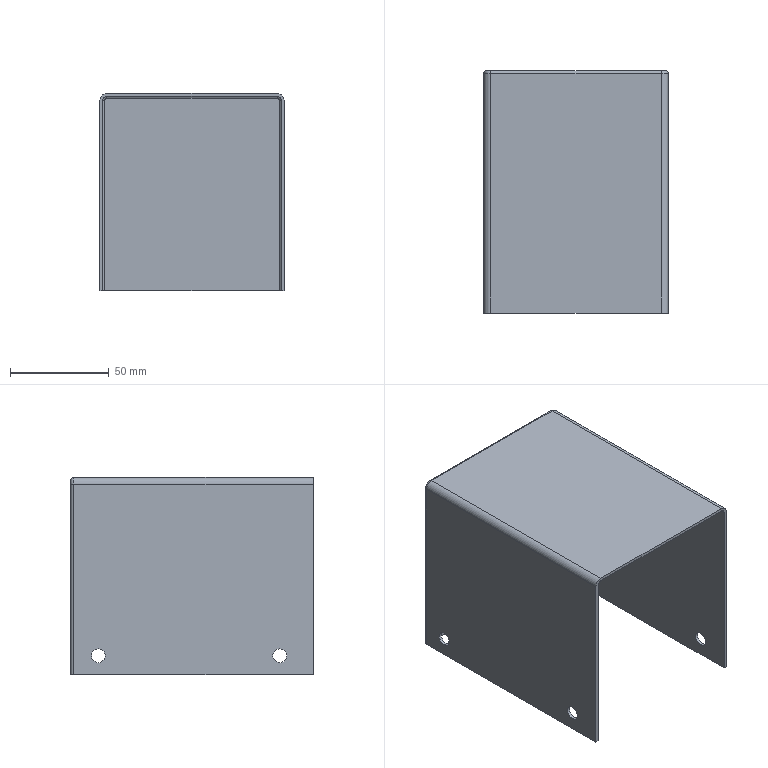Part | SolidWorks | features Fillet 4, Cut 2, Extrusion 1, ICE 1 | 1 solid | 32 faces | box 93.5 x 123 x 100 mm | volume 66221 mm3 | cylinder 18 | plane 10 | torus 4 | commonest cylinder face diameters 7 x10 2 x3 3 x3 4 x2
STEP:
#1=CARTESIAN_POINT('',(45.25,47.5,6.));
#2=VERTEX_POINT('',#1);
#3=CARTESIAN_POINT('',(45.25,47.5,13.));
#4=VERTEX_POINT('',#3);
#5=CARTESIAN_POINT('',(45.25,47.5,9.5));
#6=DIRECTION('',(-1.,0.,0.));
#7=DIRECTION('',(0.,0.,1.));
#8=AXIS2_PLACEMENT_3D('',#5,#6,#7);
#9=CIRCLE('',#8,3.5);
#10=EDGE_CURVE('',#2,#4,#9,.T.);
#11=ORIENTED_EDGE('',*,*,#10,.T.);
#12=CARTESIAN_POINT('',(46.75,47.5,13.));
#13=VERTEX_POINT('',#12);
#14=CARTESIAN_POINT('',(-46.75,47.5,13.));
#15=DIRECTION('',(1.,0.,0.));
#16=VECTOR('',#15,1000.);
#17=LINE('',#14,#16);
#18=EDGE_CURVE('',#4,#13,#17,.T.);
#19=ORIENTED_EDGE('',*,*,#18,.T.);
#20=CARTESIAN_POINT('',(46.75,47.5,6.));
#21=VERTEX_POINT('',#20);
#22=CARTESIAN_POINT('',(46.75,47.5,9.5));
#23=DIRECTION('',(1.,0.,0.));
#24=DIRECTION('',(0.,0.,-1.));
#25=AXIS2_PLACEMENT_3D('',#22,#23,#24);
#26=CIRCLE('',#25,3.5);
#27=EDGE_CURVE('',#13,#21,#26,.T.);
#28=ORIENTED_EDGE('',*,*,#27,.T.);
#29=CARTESIAN_POINT('',(-46.75,47.5,6.));
#30=DIRECTION('',(1.,0.,0.));
#31=VECTOR('',#30,1000.);
#32=LINE('',#29,#31);
#33=EDGE_CURVE('',#2,#21,#32,.T.);
#34=ORIENTED_EDGE('',*,*,#33,.F.);
#35=EDGE_LOOP('',(#11,#19,#28,#34));
#36=FACE_OUTER_BOUND('',#35,.T.);
#37=CARTESIAN_POINT('',(-46.75,47.5,9.5));
#38=DIRECTION('',(1.,0.,0.));
#39=DIRECTION('',(0.,0.,-1.));
#40=AXIS2_PLACEMENT_3D('',#37,#38,#39);
#41=CYLINDRICAL_SURFACE('',#40,3.5);
#42=ADVANCED_FACE('',(#36),#41,.F.);
#43=CARTESIAN_POINT('',(-46.75,47.5,13.));
#44=VERTEX_POINT('',#43);
#45=CARTESIAN_POINT('',(-46.75,47.5,6.));
#46=VERTEX_POINT('',#45);
#47=CARTESIAN_POINT('',(-46.75,47.5,9.5));
#48=DIRECTION('',(1.,0.,0.));
#49=DIRECTION('',(0.,0.,-1.));
#50=AXIS2_PLACEMENT_3D('',#47,#48,#49);
#51=CIRCLE('',#50,3.5);
#52=EDGE_CURVE('',#44,#46,#51,.T.);
#53=ORIENTED_EDGE('',*,*,#52,.F.);
#54=CARTESIAN_POINT('',(-45.25,47.5,13.));
#55=VERTEX_POINT('',#54);
#56=CARTESIAN_POINT('',(-46.75,47.5,13.));
#57=DIRECTION('',(1.,0.,0.));
#58=VECTOR('',#57,1000.);
#59=LINE('',#56,#58);
#60=EDGE_CURVE('',#44,#55,#59,.T.);
#61=ORIENTED_EDGE('',*,*,#60,.T.);
#62=CARTESIAN_POINT('',(-45.25,47.5,6.));
#63=VERTEX_POINT('',#62);
#64=CARTESIAN_POINT('',(-45.25,47.5,9.5));
#65=DIRECTION('',(1.,0.,0.));
#66=DIRECTION('',(0.,1.,0.));
#67=AXIS2_PLACEMENT_3D('',#64,#65,#66);
#68=CIRCLE('',#67,3.5);
#69=EDGE_CURVE('',#55,#63,#68,.T.);
#70=ORIENTED_EDGE('',*,*,#69,.T.);
#71=CARTESIAN_POINT('',(-46.75,47.5,6.));
#72=DIRECTION('',(1.,0.,0.));
#73=VECTOR('',#72,1000.);
#74=LINE('',#71,#73);
#75=EDGE_CURVE('',#46,#63,#74,.T.);
#76=ORIENTED_EDGE('',*,*,#75,.F.);
#77=EDGE_LOOP('',(#53,#61,#70,#76));
#78=FACE_OUTER_BOUND('',#77,.T.);
#79=CARTESIAN_POINT('',(-46.75,47.5,9.5));
#80=DIRECTION('',(1.,0.,0.));
#81=DIRECTION('',(0.,0.,-1.));
#82=AXIS2_PLACEMENT_3D('',#79,#80,#81);
#83=CYLINDRICAL_SURFACE('',#82,3.5);
#84=ADVANCED_FACE('',(#78),#83,.F.);
#85=CARTESIAN_POINT('',(45.25,-44.5,6.));
#86=VERTEX_POINT('',#85);
#87=CARTESIAN_POINT('',(45.25,-44.5,13.));
#88=VERTEX_POINT('',#87);
#89=CARTESIAN_POINT('',(45.25,-44.5,9.5));
#90=DIRECTION('',(-1.,0.,0.));
#91=DIRECTION('',(0.,0.,1.));
#92=AXIS2_PLACEMENT_3D('',#89,#90,#91);
#93=CIRCLE('',#92,3.5);
#94=EDGE_CURVE('',#86,#88,#93,.T.);
#95=ORIENTED_EDGE('',*,*,#94,.T.);
#96=CARTESIAN_POINT('',(46.75,-44.5,13.));
#97=VERTEX_POINT('',#96);
#98=CARTESIAN_POINT('',(-46.75,-44.5,13.));
#99=DIRECTION('',(1.,0.,0.));
#100=VECTOR('',#99,1000.);
#101=LINE('',#98,#100);
#102=EDGE_CURVE('',#88,#97,#101,.T.);
#103=ORIENTED_EDGE('',*,*,#102,.T.);
#104=CARTESIAN_POINT('',(46.75,-44.5,6.));
#105=VERTEX_POINT('',#104);
#106=CARTESIAN_POINT('',(46.75,-44.5,9.5));
#107=DIRECTION('',(1.,0.,0.));
#108=DIRECTION('',(0.,0.,-1.));
#109=AXIS2_PLACEMENT_3D('',#106,#107,#108);
#110=CIRCLE('',#109,3.5);
#111=EDGE_CURVE('',#97,#105,#110,.T.);
#112=ORIENTED_EDGE('',*,*,#111,.T.);
#113=CARTESIAN_POINT('',(-46.75,-44.5,6.));
#114=DIRECTION('',(1.,0.,0.));
#115=VECTOR('',#114,1000.);
#116=LINE('',#113,#115);
#117=EDGE_CURVE('',#86,#105,#116,.T.);
#118=ORIENTED_EDGE('',*,*,#117,.F.);
#119=EDGE_LOOP('',(#95,#103,#112,#118));
#120=FACE_OUTER_BOUND('',#119,.T.);
#121=CARTESIAN_POINT('',(-46.75,-44.5,9.5));
#122=DIRECTION('',(1.,0.,0.));
#123=DIRECTION('',(0.,0.,-1.));
#124=AXIS2_PLACEMENT_3D('',#121,#122,#123);
#125=CYLINDRICAL_SURFACE('',#124,3.5);
#126=ADVANCED_FACE('',(#120),#125,.F.);
#127=CARTESIAN_POINT('',(-46.75,-44.5,13.));
#128=VERTEX_POINT('',#127);
#129=CARTESIAN_POINT('',(-46.75,-44.5,6.));
#130=VERTEX_POINT('',#129);
#131=CARTESIAN_POINT('',(-46.75,-44.5,9.5));
#132=DIRECTION('',(1.,0.,0.));
#133=DIRECTION('',(0.,0.,-1.));
#134=AXIS2_PLACEMENT_3D('',#131,#132,#133);
#135=CIRCLE('',#134,3.5);
#136=EDGE_CURVE('',#128,#130,#135,.T.);
#137=ORIENTED_EDGE('',*,*,#136,.F.);
#138=CARTESIAN_POINT('',(-45.25,-44.5,13.));
#139=VERTEX_POINT('',#138);
#140=CARTESIAN_POINT('',(-46.75,-44.5,13.));
#141=DIRECTION('',(1.,0.,0.));
#142=VECTOR('',#141,1000.);
#143=LINE('',#140,#142);
#144=EDGE_CURVE('',#128,#139,#143,.T.);
#145=ORIENTED_EDGE('',*,*,#144,.T.);
#146=CARTESIAN_POINT('',(-45.25,-44.5,6.));
#147=VERTEX_POINT('',#146);
#148=CARTESIAN_POINT('',(-45.25,-44.5,9.5));
#149=DIRECTION('',(1.,0.,0.));
#150=DIRECTION('',(0.,1.,0.));
#151=AXIS2_PLACEMENT_3D('',#148,#149,#150);
#152=CIRCLE('',#151,3.5);
#153=EDGE_CURVE('',#139,#147,#152,.T.);
#154=ORIENTED_EDGE('',*,*,#153,.T.);
#155=CARTESIAN_POINT('',(-46.75,-44.5,6.));
#156=DIRECTION('',(1.,0.,0.));
#157=VECTOR('',#156,1000.);
#158=LINE('',#155,#157);
#159=EDGE_CURVE('',#130,#147,#158,.T.);
#160=ORIENTED_EDGE('',*,*,#159,.F.);
#161=EDGE_LOOP('',(#137,#145,#154,#160));
#162=FACE_OUTER_BOUND('',#161,.T.);
#163=CARTESIAN_POINT('',(-46.75,-44.5,9.5));
#164=DIRECTION('',(1.,0.,0.));
#165=DIRECTION('',(0.,0.,-1.));
#166=AXIS2_PLACEMENT_3D('',#163,#164,#165);
#167=CYLINDRICAL_SURFACE('',#166,3.5);
#168=ADVANCED_FACE('',(#162),#167,.F.);
#169=ORIENTED_EDGE('',*,*,#10,.F.);
#170=CARTESIAN_POINT('',(45.25,47.5,9.5));
#171=DIRECTION('',(-1.,0.,0.));
#172=DIRECTION('',(0.,0.,1.));
#173=AXIS2_PLACEMENT_3D('',#170,#171,#172);
#174=CIRCLE('',#173,3.5);
#175=EDGE_CURVE('',#4,#2,#174,.T.);
#176=ORIENTED_EDGE('',*,*,#175,.F.);
#177=EDGE_LOOP('',(#169,#176));
#178=FACE_BOUND('',#177,.T.);
#179=ORIENTED_EDGE('',*,*,#94,.F.);
#180=CARTESIAN_POINT('',(45.25,-44.5,9.5));
#181=DIRECTION('',(-1.,0.,0.));
#182=DIRECTION('',(0.,0.,1.));
#183=AXIS2_PLACEMENT_3D('',#180,#181,#182);
#184=CIRCLE('',#183,3.5);
#185=EDGE_CURVE('',#88,#86,#184,.T.);
#186=ORIENTED_EDGE('',*,*,#185,.F.);
#187=EDGE_LOOP('',(#179,#186));
#188=FACE_BOUND('',#187,.T.);
#189=CARTESIAN_POINT('',(45.25,-61.5,96.5));
#190=VERTEX_POINT('',#189);
#191=CARTESIAN_POINT('',(45.25,59.,96.5));
#192=VERTEX_POINT('',#191);
#193=CARTESIAN_POINT('',(45.25,60.,96.5));
#194=DIRECTION('',(0.,1.,0.));
#195=VECTOR('',#194,1000.);
#196=LINE('',#193,#195);
#197=EDGE_CURVE('',#190,#192,#196,.T.);
#198=ORIENTED_EDGE('',*,*,#197,.T.);
#199=CARTESIAN_POINT('',(45.25,59.,0.));
#200=VERTEX_POINT('',#199);
#201=CARTESIAN_POINT('',(45.25,59.,0.));
#202=DIRECTION('',(0.,0.,-1.));
#203=VECTOR('',#202,1000.);
#204=LINE('',#201,#203);
#205=EDGE_CURVE('',#192,#200,#204,.T.);
#206=ORIENTED_EDGE('',*,*,#205,.T.);
#207=CARTESIAN_POINT('',(45.25,-61.5,0.));
#208=VERTEX_POINT('',#207);
#209=CARTESIAN_POINT('',(45.25,60.,0.));
#210=DIRECTION('',(0.,1.,0.));
#211=VECTOR('',#210,1000.);
#212=LINE('',#209,#211);
#213=EDGE_CURVE('',#208,#200,#212,.T.);
#214=ORIENTED_EDGE('',*,*,#213,.F.);
#215=CARTESIAN_POINT('',(45.25,-61.5,0.));
#216=DIRECTION('',(0.,0.,1.));
#217=VECTOR('',#216,1000.);
#218=LINE('',#215,#217);
#219=EDGE_CURVE('',#208,#190,#218,.T.);
#220=ORIENTED_EDGE('',*,*,#219,.T.);
#221=EDGE_LOOP('',(#198,#206,#214,#220));
#222=FACE_OUTER_BOUND('',#221,.T.);
#223=CARTESIAN_POINT('',(45.25,60.,100.));
#224=DIRECTION('',(-1.,0.,0.));
#225=DIRECTION('',(0.,0.,1.));
#226=AXIS2_PLACEMENT_3D('',#223,#224,#225);
#227=PLANE('',#226);
#228=ADVANCED_FACE('',(#178,#188,#222),#227,.T.);
#229=CARTESIAN_POINT('',(44.25,60.,0.));
#230=VERTEX_POINT('',#229);
#231=CARTESIAN_POINT('',(-44.25,60.,0.));
#232=VERTEX_POINT('',#231);
#233=CARTESIAN_POINT('',(-45.25,60.,0.));
#234=DIRECTION('',(-1.,0.,0.));
#235=VECTOR('',#234,1000.);
#236=LINE('',#233,#235);
#237=EDGE_CURVE('',#230,#232,#236,.T.);
#238=ORIENTED_EDGE('',*,*,#237,.F.);
#239=CARTESIAN_POINT('',(44.25,60.,96.5));
#240=VERTEX_POINT('',#239);
#241=CARTESIAN_POINT('',(44.25,60.,96.5));
#242=DIRECTION('',(0.,0.,1.));
#243=VECTOR('',#242,1000.);
#244=LINE('',#241,#243);
#245=EDGE_CURVE('',#230,#240,#244,.T.);
#246=ORIENTED_EDGE('',*,*,#245,.T.);
#247=CARTESIAN_POINT('',(43.25,60.,97.5));
#248=VERTEX_POINT('',#247);
#249=CARTESIAN_POINT('',(43.25,60.,96.5));
#250=DIRECTION('',(0.,-1.,0.));
#251=DIRECTION('',(0.,0.,-1.));
#252=AXIS2_PLACEMENT_3D('',#249,#250,#251);
#253=CIRCLE('',#252,1.);
#254=EDGE_CURVE('',#240,#248,#253,.T.);
#255=ORIENTED_EDGE('',*,*,#254,.T.);
#256=CARTESIAN_POINT('',(-43.25,60.,97.5));
#257=VERTEX_POINT('',#256);
#258=CARTESIAN_POINT('',(-45.25,60.,97.5));
#259=DIRECTION('',(-1.,0.,0.));
#260=VECTOR('',#259,1000.);
#261=LINE('',#258,#260);
#262=EDGE_CURVE('',#248,#257,#261,.T.);
#263=ORIENTED_EDGE('',*,*,#262,.T.);
#264=CARTESIAN_POINT('',(-44.25,60.,96.5));
#265=VERTEX_POINT('',#264);
#266=CARTESIAN_POINT('',(-43.25,60.,96.5));
#267=DIRECTION('',(0.,-1.,0.));
#268=DIRECTION('',(0.,0.,-1.));
#269=AXIS2_PLACEMENT_3D('',#266,#267,#268);
#270=CIRCLE('',#269,1.);
#271=EDGE_CURVE('',#257,#265,#270,.T.);
#272=ORIENTED_EDGE('',*,*,#271,.T.);
#273=CARTESIAN_POINT('',(-44.25,60.,0.));
#274=DIRECTION('',(0.,0.,-1.));
#275=VECTOR('',#274,1000.);
#276=LINE('',#273,#275);
#277=EDGE_CURVE('',#265,#232,#276,.T.);
#278=ORIENTED_EDGE('',*,*,#277,.T.);
#279=EDGE_LOOP('',(#238,#246,#255,#263,#272,#278));
#280=FACE_OUTER_BOUND('',#279,.T.);
#281=CARTESIAN_POINT('',(-45.25,60.,100.));
#282=DIRECTION('',(0.,-1.,0.));
#283=DIRECTION('',(0.,0.,-1.));
#284=AXIS2_PLACEMENT_3D('',#281,#282,#283);
#285=PLANE('',#284);
#286=ADVANCED_FACE('',(#280),#285,.T.);
#287=CARTESIAN_POINT('',(-45.25,47.5,9.5));
#288=DIRECTION('',(1.,0.,0.));
#289=DIRECTION('',(0.,1.,0.));
#290=AXIS2_PLACEMENT_3D('',#287,#288,#289);
#291=CIRCLE('',#290,3.5);
#292=EDGE_CURVE('',#63,#55,#291,.T.);
#293=ORIENTED_EDGE('',*,*,#292,.F.);
#294=ORIENTED_EDGE('',*,*,#69,.F.);
#295=EDGE_LOOP('',(#293,#294));
#296=FACE_BOUND('',#295,.T.);
#297=CARTESIAN_POINT('',(-45.25,-44.5,9.5));
#298=DIRECTION('',(1.,0.,0.));
#299=DIRECTION('',(0.,1.,0.));
#300=AXIS2_PLACEMENT_3D('',#297,#298,#299);
#301=CIRCLE('',#300,3.5);
#302=EDGE_CURVE('',#147,#139,#301,.T.);
#303=ORIENTED_EDGE('',*,*,#302,.F.);
#304=ORIENTED_EDGE('',*,*,#153,.F.);
#305=EDGE_LOOP('',(#303,#304));
#306=FACE_BOUND('',#305,.T.);
#307=CARTESIAN_POINT('',(-45.25,59.,0.));
#308=VERTEX_POINT('',#307);
#309=CARTESIAN_POINT('',(-45.25,-61.5,0.));
#310=VERTEX_POINT('',#309);
#311=CARTESIAN_POINT('',(-45.25,60.,0.));
#312=DIRECTION('',(0.,-1.,0.));
#313=VECTOR('',#312,1000.);
#314=LINE('',#311,#313);
#315=EDGE_CURVE('',#308,#310,#314,.T.);
#316=ORIENTED_EDGE('',*,*,#315,.F.);
#317=CARTESIAN_POINT('',(-45.25,59.,96.5));
#318=VERTEX_POINT('',#317);
#319=CARTESIAN_POINT('',(-45.25,59.,96.5));
#320=DIRECTION('',(0.,0.,1.));
#321=VECTOR('',#320,1000.);
#322=LINE('',#319,#321);
#323=EDGE_CURVE('',#308,#318,#322,.T.);
#324=ORIENTED_EDGE('',*,*,#323,.T.);
#325=CARTESIAN_POINT('',(-45.25,-61.5,96.5));
#326=VERTEX_POINT('',#325);
#327=CARTESIAN_POINT('',(-45.25,60.,96.5));
#328=DIRECTION('',(0.,-1.,0.));
#329=VECTOR('',#328,1000.);
#330=LINE('',#327,#329);
#331=EDGE_CURVE('',#318,#326,#330,.T.);
#332=ORIENTED_EDGE('',*,*,#331,.T.);
#333=CARTESIAN_POINT('',(-45.25,-61.5,0.));
#334=DIRECTION('',(0.,0.,-1.));
#335=VECTOR('',#334,1000.);
#336=LINE('',#333,#335);
#337=EDGE_CURVE('',#326,#310,#336,.T.);
#338=ORIENTED_EDGE('',*,*,#337,.T.);
#339=EDGE_LOOP('',(#316,#324,#332,#338));
#340=FACE_OUTER_BOUND('',#339,.T.);
#341=CARTESIAN_POINT('',(-45.25,60.,100.));
#342=DIRECTION('',(1.,0.,0.));
#343=DIRECTION('',(0.,1.,0.));
#344=AXIS2_PLACEMENT_3D('',#341,#342,#343);
#345=PLANE('',#344);
#346=ADVANCED_FACE('',(#296,#306,#340),#345,.T.);
#347=CARTESIAN_POINT('',(43.25,-61.5,100.));
#348=VERTEX_POINT('',#347);
#349=CARTESIAN_POINT('',(43.25,60.,100.));
#350=VERTEX_POINT('',#349);
#351=CARTESIAN_POINT('',(43.25,61.5,100.));
#352=DIRECTION('',(0.,1.,0.));
#353=VECTOR('',#352,1000.);
#354=LINE('',#351,#353);
#355=EDGE_CURVE('',#348,#350,#354,.T.);
#356=ORIENTED_EDGE('',*,*,#355,.T.);
#357=CARTESIAN_POINT('',(-43.25,60.,100.));
#358=VERTEX_POINT('',#357);
#359=CARTESIAN_POINT('',(-43.25,60.,100.));
#360=DIRECTION('',(-1.,0.,0.));
#361=VECTOR('',#360,1000.);
#362=LINE('',#359,#361);
#363=EDGE_CURVE('',#350,#358,#362,.T.);
#364=ORIENTED_EDGE('',*,*,#363,.T.);
#365=CARTESIAN_POINT('',(-43.25,-61.5,100.));
#366=VERTEX_POINT('',#365);
#367=CARTESIAN_POINT('',(-43.25,-61.5,100.));
#368=DIRECTION('',(0.,-1.,0.));
#369=VECTOR('',#368,1000.);
#370=LINE('',#367,#369);
#371=EDGE_CURVE('',#358,#366,#370,.T.);
#372=ORIENTED_EDGE('',*,*,#371,.T.);
#373=CARTESIAN_POINT('',(-46.75,-61.5,100.));
#374=DIRECTION('',(1.,0.,0.));
#375=VECTOR('',#374,1000.);
#376=LINE('',#373,#375);
#377=EDGE_CURVE('',#366,#348,#376,.T.);
#378=ORIENTED_EDGE('',*,*,#377,.T.);
#379=EDGE_LOOP('',(#356,#364,#372,#378));
#380=FACE_OUTER_BOUND('',#379,.T.);
#381=CARTESIAN_POINT('',(0.,0.,100.));
#382=DIRECTION('',(0.,0.,1.));
#383=DIRECTION('',(1.,0.,0.));
#384=AXIS2_PLACEMENT_3D('',#381,#382,#383);
#385=PLANE('',#384);
#386=ADVANCED_FACE('',(#380),#385,.T.);
#387=CARTESIAN_POINT('',(45.25,61.5,0.));
#388=VERTEX_POINT('',#387);
#389=CARTESIAN_POINT('',(-45.25,61.5,0.));
#390=VERTEX_POINT('',#389);
#391=CARTESIAN_POINT('',(-46.75,61.5,0.));
#392=DIRECTION('',(-1.,0.,0.));
#393=VECTOR('',#392,1000.);
#394=LINE('',#391,#393);
#395=EDGE_CURVE('',#388,#390,#394,.T.);
#396=ORIENTED_EDGE('',*,*,#395,.F.);
#397=CARTESIAN_POINT('',(46.75,60.,0.));
#398=VERTEX_POINT('',#397);
#399=CARTESIAN_POINT('',(45.25,60.,0.));
#400=DIRECTION('',(0.,0.,-1.));
#401=DIRECTION('',(1.,0.,0.));
#402=AXIS2_PLACEMENT_3D('',#399,#400,#401);
#403=CIRCLE('',#402,1.5);
#404=EDGE_CURVE('',#388,#398,#403,.T.);
#405=ORIENTED_EDGE('',*,*,#404,.T.);
#406=CARTESIAN_POINT('',(46.75,-61.5,0.));
#407=VERTEX_POINT('',#406);
#408=CARTESIAN_POINT('',(46.75,61.5,0.));
#409=DIRECTION('',(0.,1.,0.));
#410=VECTOR('',#409,1000.);
#411=LINE('',#408,#410);
#412=EDGE_CURVE('',#407,#398,#411,.T.);
#413=ORIENTED_EDGE('',*,*,#412,.F.);
#414=CARTESIAN_POINT('',(-46.75,-61.5,0.));
#415=DIRECTION('',(1.,0.,0.));
#416=VECTOR('',#415,1000.);
#417=LINE('',#414,#416);
#418=EDGE_CURVE('',#208,#407,#417,.T.);
#419=ORIENTED_EDGE('',*,*,#418,.F.);
#420=ORIENTED_EDGE('',*,*,#213,.T.);
#421=CARTESIAN_POINT('',(44.25,59.,0.));
#422=DIRECTION('',(0.,0.,1.));
#423=DIRECTION('',(1.,0.,0.));
#424=AXIS2_PLACEMENT_3D('',#421,#422,#423);
#425=CIRCLE('',#424,1.);
#426=EDGE_CURVE('',#200,#230,#425,.T.);
#427=ORIENTED_EDGE('',*,*,#426,.T.);
#428=ORIENTED_EDGE('',*,*,#237,.T.);
#429=CARTESIAN_POINT('',(-44.25,59.,0.));
#430=DIRECTION('',(0.,0.,1.));
#431=DIRECTION('',(1.,0.,0.));
#432=AXIS2_PLACEMENT_3D('',#429,#430,#431);
#433=CIRCLE('',#432,1.);
#434=EDGE_CURVE('',#232,#308,#433,.T.);
#435=ORIENTED_EDGE('',*,*,#434,.T.);
#436=ORIENTED_EDGE('',*,*,#315,.T.);
#437=CARTESIAN_POINT('',(-46.75,-61.5,0.));
#438=VERTEX_POINT('',#437);
#439=CARTESIAN_POINT('',(-46.75,-61.5,0.));
#440=DIRECTION('',(1.,0.,0.));
#441=VECTOR('',#440,1000.);
#442=LINE('',#439,#441);
#443=EDGE_CURVE('',#438,#310,#442,.T.);
#444=ORIENTED_EDGE('',*,*,#443,.F.);
#445=CARTESIAN_POINT('',(-46.75,60.,0.));
#446=VERTEX_POINT('',#445);
#447=CARTESIAN_POINT('',(-46.75,61.5,0.));
#448=DIRECTION('',(0.,-1.,0.));
#449=VECTOR('',#448,1000.);
#450=LINE('',#447,#449);
#451=EDGE_CURVE('',#446,#438,#450,.T.);
#452=ORIENTED_EDGE('',*,*,#451,.F.);
#453=CARTESIAN_POINT('',(-45.25,60.,0.));
#454=DIRECTION('',(0.,0.,-1.));
#455=DIRECTION('',(1.,0.,0.));
#456=AXIS2_PLACEMENT_3D('',#453,#454,#455);
#457=CIRCLE('',#456,1.5);
#458=EDGE_CURVE('',#446,#390,#457,.T.);
#459=ORIENTED_EDGE('',*,*,#458,.T.);
#460=EDGE_LOOP('',(#396,#405,#413,#419,#420,#427,#428,#435,#436,#444,#452,#459));
#461=FACE_OUTER_BOUND('',#460,.T.);
#462=CARTESIAN_POINT('',(0.,0.,0.));
#463=DIRECTION('',(0.,0.,1.));
#464=DIRECTION('',(1.,0.,0.));
#465=AXIS2_PLACEMENT_3D('',#462,#463,#464);
#466=PLANE('',#465);
#467=ADVANCED_FACE('',(#461),#466,.F.);
#468=CARTESIAN_POINT('',(46.75,47.5,9.5));
#469=DIRECTION('',(1.,0.,0.));
#470=DIRECTION('',(0.,0.,-1.));
#471=AXIS2_PLACEMENT_3D('',#468,#469,#470);
#472=CIRCLE('',#471,3.5);
#473=EDGE_CURVE('',#21,#13,#472,.T.);
#474=ORIENTED_EDGE('',*,*,#473,.F.);
#475=ORIENTED_EDGE('',*,*,#27,.F.);
#476=EDGE_LOOP('',(#474,#475));
#477=FACE_BOUND('',#476,.T.);
#478=CARTESIAN_POINT('',(46.75,-44.5,9.5));
#479=DIRECTION('',(1.,0.,0.));
#480=DIRECTION('',(0.,0.,-1.));
#481=AXIS2_PLACEMENT_3D('',#478,#479,#480);
#482=CIRCLE('',#481,3.5);
#483=EDGE_CURVE('',#105,#97,#482,.T.);
#484=ORIENTED_EDGE('',*,*,#483,.F.);
#485=ORIENTED_EDGE('',*,*,#111,.F.);
#486=EDGE_LOOP('',(#484,#485));
#487=FACE_BOUND('',#486,.T.);
#488=ORIENTED_EDGE('',*,*,#412,.T.);
#489=CARTESIAN_POINT('',(46.75,60.,96.5));
#490=VERTEX_POINT('',#489);
#491=CARTESIAN_POINT('',(46.75,60.,100.));
#492=DIRECTION('',(0.,0.,1.));
#493=VECTOR('',#492,1000.);
#494=LINE('',#491,#493);
#495=EDGE_CURVE('',#398,#490,#494,.T.);
#496=ORIENTED_EDGE('',*,*,#495,.T.);
#497=CARTESIAN_POINT('',(46.75,-61.5,96.5));
#498=VERTEX_POINT('',#497);
#499=CARTESIAN_POINT('',(46.75,-61.5,96.5));
#500=DIRECTION('',(0.,-1.,0.));
#501=VECTOR('',#500,1000.);
#502=LINE('',#499,#501);
#503=EDGE_CURVE('',#490,#498,#502,.T.);
#504=ORIENTED_EDGE('',*,*,#503,.T.);
#505=CARTESIAN_POINT('',(46.75,-61.5,100.));
#506=DIRECTION('',(0.,0.,-1.));
#507=VECTOR('',#506,1000.);
#508=LINE('',#505,#507);
#509=EDGE_CURVE('',#498,#407,#508,.T.);
#510=ORIENTED_EDGE('',*,*,#509,.T.);
#511=EDGE_LOOP('',(#488,#496,#504,#510));
#512=FACE_OUTER_BOUND('',#511,.T.);
#513=CARTESIAN_POINT('',(46.75,61.5,100.));
#514=DIRECTION('',(-1.,0.,0.));
#515=DIRECTION('',(0.,0.,1.));
#516=AXIS2_PLACEMENT_3D('',#513,#514,#515);
#517=PLANE('',#516);
#518=ADVANCED_FACE('',(#477,#487,#512),#517,.F.);
#519=CARTESIAN_POINT('',(43.25,61.5,98.5));
#520=VERTEX_POINT('',#519);
#521=CARTESIAN_POINT('',(45.25,61.5,96.5));
#522=VERTEX_POINT('',#521);
#523=CARTESIAN_POINT('',(43.25,61.5,96.5));
#524=DIRECTION('',(0.,1.,0.));
#525=DIRECTION('',(0.,0.,-1.));
#526=AXIS2_PLACEMENT_3D('',#523,#524,#525);
#527=CIRCLE('',#526,2.);
#528=EDGE_CURVE('',#520,#522,#527,.T.);
#529=ORIENTED_EDGE('',*,*,#528,.T.);
#530=CARTESIAN_POINT('',(45.25,61.5,100.));
#531=DIRECTION('',(0.,0.,-1.));
#532=VECTOR('',#531,1000.);
#533=LINE('',#530,#532);
#534=EDGE_CURVE('',#522,#388,#533,.T.);
#535=ORIENTED_EDGE('',*,*,#534,.T.);
#536=ORIENTED_EDGE('',*,*,#395,.T.);
#537=CARTESIAN_POINT('',(-45.25,61.5,96.5));
#538=VERTEX_POINT('',#537);
#539=CARTESIAN_POINT('',(-45.25,61.5,100.));
#540=DIRECTION('',(0.,0.,1.));
#541=VECTOR('',#540,1000.);
#542=LINE('',#539,#541);
#543=EDGE_CURVE('',#390,#538,#542,.T.);
#544=ORIENTED_EDGE('',*,*,#543,.T.);
#545=CARTESIAN_POINT('',(-43.25,61.5,98.5));
#546=VERTEX_POINT('',#545);
#547=CARTESIAN_POINT('',(-43.25,61.5,96.5));
#548=DIRECTION('',(0.,1.,0.));
#549=DIRECTION('',(0.,0.,-1.));
#550=AXIS2_PLACEMENT_3D('',#547,#548,#549);
#551=CIRCLE('',#550,2.);
#552=EDGE_CURVE('',#538,#546,#551,.T.);
#553=ORIENTED_EDGE('',*,*,#552,.T.);
#554=CARTESIAN_POINT('',(43.25,61.5,98.5));
#555=DIRECTION('',(1.,0.,0.));
#556=VECTOR('',#555,1000.);
#557=LINE('',#554,#556);
#558=EDGE_CURVE('',#546,#520,#557,.T.);
#559=ORIENTED_EDGE('',*,*,#558,.T.);
#560=EDGE_LOOP('',(#529,#535,#536,#544,#553,#559));
#561=FACE_OUTER_BOUND('',#560,.T.);
#562=CARTESIAN_POINT('',(-46.75,61.5,100.));
#563=DIRECTION('',(0.,-1.,0.));
#564=DIRECTION('',(0.,0.,-1.));
#565=AXIS2_PLACEMENT_3D('',#562,#563,#564);
#566=PLANE('',#565);
#567=ADVANCED_FACE('',(#561),#566,.F.);
#568=CARTESIAN_POINT('',(-46.75,47.5,9.5));
#569=DIRECTION('',(1.,0.,0.));
#570=DIRECTION('',(0.,0.,-1.));
#571=AXIS2_PLACEMENT_3D('',#568,#569,#570);
#572=CIRCLE('',#571,3.5);
#573=EDGE_CURVE('',#46,#44,#572,.T.);
#574=ORIENTED_EDGE('',*,*,#573,.T.);
#575=ORIENTED_EDGE('',*,*,#52,.T.);
#576=EDGE_LOOP('',(#574,#575));
#577=FACE_BOUND('',#576,.T.);
#578=CARTESIAN_POINT('',(-46.75,-44.5,9.5));
#579=DIRECTION('',(1.,0.,0.));
#580=DIRECTION('',(0.,0.,-1.));
#581=AXIS2_PLACEMENT_3D('',#578,#579,#580);
#582=CIRCLE('',#581,3.5);
#583=EDGE_CURVE('',#130,#128,#582,.T.);
#584=ORIENTED_EDGE('',*,*,#583,.T.);
#585=ORIENTED_EDGE('',*,*,#136,.T.);
#586=EDGE_LOOP('',(#584,#585));
#587=FACE_BOUND('',#586,.T.);
#588=CARTESIAN_POINT('',(-46.75,-61.5,96.5));
#589=VERTEX_POINT('',#588);
#590=CARTESIAN_POINT('',(-46.75,60.,96.5));
#591=VERTEX_POINT('',#590);
#592=CARTESIAN_POINT('',(-46.75,61.5,96.5));
#593=DIRECTION('',(0.,1.,0.));
#594=VECTOR('',#593,1000.);
#595=LINE('',#592,#594);
#596=EDGE_CURVE('',#589,#591,#595,.T.);
#597=ORIENTED_EDGE('',*,*,#596,.T.);
#598=CARTESIAN_POINT('',(-46.75,60.,100.));
#599=DIRECTION('',(0.,0.,-1.));
#600=VECTOR('',#599,1000.);
#601=LINE('',#598,#600);
#602=EDGE_CURVE('',#591,#446,#601,.T.);
#603=ORIENTED_EDGE('',*,*,#602,.T.);
#604=ORIENTED_EDGE('',*,*,#451,.T.);
#605=CARTESIAN_POINT('',(-46.75,-61.5,100.));
#606=DIRECTION('',(0.,0.,-1.));
#607=VECTOR('',#606,1000.);
#608=LINE('',#605,#607);
#609=EDGE_CURVE('',#589,#438,#608,.T.);
#610=ORIENTED_EDGE('',*,*,#609,.F.);
#611=EDGE_LOOP('',(#597,#603,#604,#610));
#612=FACE_OUTER_BOUND('',#611,.T.);
#613=CARTESIAN_POINT('',(-46.75,61.5,100.));
#614=DIRECTION('',(1.,0.,0.));
#615=DIRECTION('',(0.,0.,-1.));
#616=AXIS2_PLACEMENT_3D('',#613,#614,#615);
#617=PLANE('',#616);
#618=ADVANCED_FACE('',(#577,#587,#612),#617,.F.);
#619=ORIENTED_EDGE('',*,*,#509,.F.);
#620=CARTESIAN_POINT('',(43.25,-61.5,96.5));
#621=DIRECTION('',(0.,-1.,0.));
#622=DIRECTION('',(0.,0.,1.));
#623=AXIS2_PLACEMENT_3D('',#620,#621,#622);
#624=CIRCLE('',#623,3.5);
#625=EDGE_CURVE('',#498,#348,#624,.T.);
#626=ORIENTED_EDGE('',*,*,#625,.T.);
#627=ORIENTED_EDGE('',*,*,#377,.F.);
#628=CARTESIAN_POINT('',(-43.25,-61.5,96.5));
#629=DIRECTION('',(0.,-1.,0.));
#630=DIRECTION('',(0.,0.,1.));
#631=AXIS2_PLACEMENT_3D('',#628,#629,#630);
#632=CIRCLE('',#631,3.5);
#633=EDGE_CURVE('',#366,#589,#632,.T.);
#634=ORIENTED_EDGE('',*,*,#633,.T.);
#635=ORIENTED_EDGE('',*,*,#609,.T.);
#636=ORIENTED_EDGE('',*,*,#443,.T.);
#637=ORIENTED_EDGE('',*,*,#337,.F.);
#638=CARTESIAN_POINT('',(-43.25,-61.5,98.5));
#639=VERTEX_POINT('',#638);
#640=CARTESIAN_POINT('',(-43.25,-61.5,96.5));
#641=DIRECTION('',(0.,1.,0.));
#642=DIRECTION('',(0.,0.,1.));
#643=AXIS2_PLACEMENT_3D('',#640,#641,#642);
#644=CIRCLE('',#643,2.);
#645=EDGE_CURVE('',#326,#639,#644,.T.);
#646=ORIENTED_EDGE('',*,*,#645,.T.);
#647=CARTESIAN_POINT('',(43.25,-61.5,98.5));
#648=VERTEX_POINT('',#647);
#649=CARTESIAN_POINT('',(-45.25,-61.5,98.5));
#650=DIRECTION('',(-1.,0.,0.));
#651=VECTOR('',#650,1000.);
#652=LINE('',#649,#651);
#653=EDGE_CURVE('',#648,#639,#652,.T.);
#654=ORIENTED_EDGE('',*,*,#653,.F.);
#655=CARTESIAN_POINT('',(43.25,-61.5,96.5));
#656=DIRECTION('',(0.,1.,0.));
#657=DIRECTION('',(0.,0.,1.));
#658=AXIS2_PLACEMENT_3D('',#655,#656,#657);
#659=CIRCLE('',#658,2.);
#660=EDGE_CURVE('',#648,#190,#659,.T.);
#661=ORIENTED_EDGE('',*,*,#660,.T.);
#662=ORIENTED_EDGE('',*,*,#219,.F.);
#663=ORIENTED_EDGE('',*,*,#418,.T.);
#664=EDGE_LOOP('',(#619,#626,#627,#634,#635,#636,#637,#646,#654,#661,#662,#663));
#665=FACE_OUTER_BOUND('',#664,.T.);
#666=CARTESIAN_POINT('',(-46.75,-61.5,100.));
#667=DIRECTION('',(0.,1.,0.));
#668=DIRECTION('',(0.,0.,1.));
#669=AXIS2_PLACEMENT_3D('',#666,#667,#668);
#670=PLANE('',#669);
#671=ADVANCED_FACE('',(#665),#670,.F.);
#672=CARTESIAN_POINT('',(-43.25,59.,98.5));
#673=VERTEX_POINT('',#672);
#674=CARTESIAN_POINT('',(-43.25,0.,98.5));
#675=DIRECTION('',(0.,1.,0.));
#676=VECTOR('',#675,1000.);
#677=LINE('',#674,#676);
#678=EDGE_CURVE('',#639,#673,#677,.T.);
#679=ORIENTED_EDGE('',*,*,#678,.T.);
#680=CARTESIAN_POINT('',(43.25,59.,98.5));
#681=VERTEX_POINT('',#680);
#682=CARTESIAN_POINT('',(0.,59.,98.5));
#683=DIRECTION('',(1.,0.,0.));
#684=VECTOR('',#683,1000.);
#685=LINE('',#682,#684);
#686=EDGE_CURVE('',#673,#681,#685,.T.);
#687=ORIENTED_EDGE('',*,*,#686,.T.);
#688=CARTESIAN_POINT('',(43.25,0.,98.5));
#689=DIRECTION('',(0.,-1.,0.));
#690=VECTOR('',#689,1000.);
#691=LINE('',#688,#690);
#692=EDGE_CURVE('',#681,#648,#691,.T.);
#693=ORIENTED_EDGE('',*,*,#692,.T.);
#694=ORIENTED_EDGE('',*,*,#653,.T.);
#695=EDGE_LOOP('',(#679,#687,#693,#694));
#696=FACE_OUTER_BOUND('',#695,.T.);
#697=CARTESIAN_POINT('',(0.,0.,98.5));
#698=DIRECTION('',(0.,0.,1.));
#699=DIRECTION('',(1.,0.,0.));
#700=AXIS2_PLACEMENT_3D('',#697,#698,#699);
#701=PLANE('',#700);
#702=ADVANCED_FACE('',(#696),#701,.F.);
#703=ORIENTED_EDGE('',*,*,#144,.F.);
#704=ORIENTED_EDGE('',*,*,#583,.F.);
#705=ORIENTED_EDGE('',*,*,#159,.T.);
#706=ORIENTED_EDGE('',*,*,#302,.T.);
#707=EDGE_LOOP('',(#703,#704,#705,#706));
#708=FACE_OUTER_BOUND('',#707,.T.);
#709=CARTESIAN_POINT('',(-46.75,-44.5,9.5));
#710=DIRECTION('',(1.,0.,0.));
#711=DIRECTION('',(0.,0.,-1.));
#712=AXIS2_PLACEMENT_3D('',#709,#710,#711);
#713=CYLINDRICAL_SURFACE('',#712,3.5);
#714=ADVANCED_FACE('',(#708),#713,.F.);
#715=ORIENTED_EDGE('',*,*,#102,.F.);
#716=ORIENTED_EDGE('',*,*,#185,.T.);
#717=ORIENTED_EDGE('',*,*,#117,.T.);
#718=ORIENTED_EDGE('',*,*,#483,.T.);
#719=EDGE_LOOP('',(#715,#716,#717,#718));
#720=FACE_OUTER_BOUND('',#719,.T.);
#721=CARTESIAN_POINT('',(-46.75,-44.5,9.5));
#722=DIRECTION('',(1.,0.,0.));
#723=DIRECTION('',(0.,0.,-1.));
#724=AXIS2_PLACEMENT_3D('',#721,#722,#723);
#725=CYLINDRICAL_SURFACE('',#724,3.5);
#726=ADVANCED_FACE('',(#720),#725,.F.);
#727=ORIENTED_EDGE('',*,*,#60,.F.);
#728=ORIENTED_EDGE('',*,*,#573,.F.);
#729=ORIENTED_EDGE('',*,*,#75,.T.);
#730=ORIENTED_EDGE('',*,*,#292,.T.);
#731=EDGE_LOOP('',(#727,#728,#729,#730));
#732=FACE_OUTER_BOUND('',#731,.T.);
#733=CARTESIAN_POINT('',(-46.75,47.5,9.5));
#734=DIRECTION('',(1.,0.,0.));
#735=DIRECTION('',(0.,0.,-1.));
#736=AXIS2_PLACEMENT_3D('',#733,#734,#735);
#737=CYLINDRICAL_SURFACE('',#736,3.5);
#738=ADVANCED_FACE('',(#732),#737,.F.);
#739=ORIENTED_EDGE('',*,*,#18,.F.);
#740=ORIENTED_EDGE('',*,*,#175,.T.);
#741=ORIENTED_EDGE('',*,*,#33,.T.);
#742=ORIENTED_EDGE('',*,*,#473,.T.);
#743=EDGE_LOOP('',(#739,#740,#741,#742));
#744=FACE_OUTER_BOUND('',#743,.T.);
#745=CARTESIAN_POINT('',(-46.75,47.5,9.5));
#746=DIRECTION('',(1.,0.,0.));
#747=DIRECTION('',(0.,0.,-1.));
#748=AXIS2_PLACEMENT_3D('',#745,#746,#747);
#749=CYLINDRICAL_SURFACE('',#748,3.5);
#750=ADVANCED_FACE('',(#744),#749,.F.);
#751=ORIENTED_EDGE('',*,*,#331,.F.);
#752=CARTESIAN_POINT('',(-43.25,59.,96.5));
#753=DIRECTION('',(0.,1.,0.));
#754=DIRECTION('',(0.,0.,-1.));
#755=AXIS2_PLACEMENT_3D('',#752,#753,#754);
#756=CIRCLE('',#755,2.);
#757=EDGE_CURVE('',#318,#673,#756,.T.);
#758=ORIENTED_EDGE('',*,*,#757,.T.);
#759=ORIENTED_EDGE('',*,*,#678,.F.);
#760=ORIENTED_EDGE('',*,*,#645,.F.);
#761=EDGE_LOOP('',(#751,#758,#759,#760));
#762=FACE_OUTER_BOUND('',#761,.T.);
#763=CARTESIAN_POINT('',(-43.25,60.,96.5));
#764=DIRECTION('',(0.,-1.,0.));
#765=DIRECTION('',(1.,0.,0.));
#766=AXIS2_PLACEMENT_3D('',#763,#764,#765);
#767=CYLINDRICAL_SURFACE('',#766,2.);
#768=ADVANCED_FACE('',(#762),#767,.F.);
#769=ORIENTED_EDGE('',*,*,#692,.F.);
#770=CARTESIAN_POINT('',(43.25,59.,96.5));
#771=DIRECTION('',(0.,1.,0.));
#772=DIRECTION('',(0.,0.,-1.));
#773=AXIS2_PLACEMENT_3D('',#770,#771,#772);
#774=CIRCLE('',#773,2.);
#775=EDGE_CURVE('',#681,#192,#774,.T.);
#776=ORIENTED_EDGE('',*,*,#775,.T.);
#777=ORIENTED_EDGE('',*,*,#197,.F.);
#778=ORIENTED_EDGE('',*,*,#660,.F.);
#779=EDGE_LOOP('',(#769,#776,#777,#778));
#780=FACE_OUTER_BOUND('',#779,.T.);
#781=CARTESIAN_POINT('',(43.25,60.,96.5));
#782=DIRECTION('',(0.,1.,0.));
#783=DIRECTION('',(0.,0.,1.));
#784=AXIS2_PLACEMENT_3D('',#781,#782,#783);
#785=CYLINDRICAL_SURFACE('',#784,2.);
#786=ADVANCED_FACE('',(#780),#785,.F.);
#787=ORIENTED_EDGE('',*,*,#503,.F.);
#788=CARTESIAN_POINT('',(43.25,60.,96.5));
#789=DIRECTION('',(0.,-1.,0.));
#790=DIRECTION('',(0.,0.,-1.));
#791=AXIS2_PLACEMENT_3D('',#788,#789,#790);
#792=CIRCLE('',#791,3.5);
#793=EDGE_CURVE('',#490,#350,#792,.T.);
#794=ORIENTED_EDGE('',*,*,#793,.T.);
#795=ORIENTED_EDGE('',*,*,#355,.F.);
#796=ORIENTED_EDGE('',*,*,#625,.F.);
#797=EDGE_LOOP('',(#787,#794,#795,#796));
#798=FACE_OUTER_BOUND('',#797,.T.);
#799=CARTESIAN_POINT('',(43.25,0.,96.5));
#800=DIRECTION('',(0.,-1.,0.));
#801=DIRECTION('',(0.,0.,-1.));
#802=AXIS2_PLACEMENT_3D('',#799,#800,#801);
#803=CYLINDRICAL_SURFACE('',#802,3.5);
#804=ADVANCED_FACE('',(#798),#803,.T.);
#805=ORIENTED_EDGE('',*,*,#371,.F.);
#806=CARTESIAN_POINT('',(-43.25,60.,96.5));
#807=DIRECTION('',(0.,-1.,0.));
#808=DIRECTION('',(0.,0.,-1.));
#809=AXIS2_PLACEMENT_3D('',#806,#807,#808);
#810=CIRCLE('',#809,3.5);
#811=EDGE_CURVE('',#358,#591,#810,.T.);
#812=ORIENTED_EDGE('',*,*,#811,.T.);
#813=ORIENTED_EDGE('',*,*,#596,.F.);
#814=ORIENTED_EDGE('',*,*,#633,.F.);
#815=EDGE_LOOP('',(#805,#812,#813,#814));
#816=FACE_OUTER_BOUND('',#815,.T.);
#817=CARTESIAN_POINT('',(-43.25,0.,96.5));
#818=DIRECTION('',(0.,1.,0.));
#819=DIRECTION('',(0.,0.,1.));
#820=AXIS2_PLACEMENT_3D('',#817,#818,#819);
#821=CYLINDRICAL_SURFACE('',#820,3.5);
#822=ADVANCED_FACE('',(#816),#821,.T.);
#823=ORIENTED_EDGE('',*,*,#434,.F.);
#824=ORIENTED_EDGE('',*,*,#277,.F.);
#825=CARTESIAN_POINT('',(-44.25,59.,96.5));
#826=DIRECTION('',(0.,0.,-1.));
#827=DIRECTION('',(-1.,0.,0.));
#828=AXIS2_PLACEMENT_3D('',#825,#826,#827);
#829=CIRCLE('',#828,1.);
#830=EDGE_CURVE('',#318,#265,#829,.T.);
#831=ORIENTED_EDGE('',*,*,#830,.F.);
#832=ORIENTED_EDGE('',*,*,#323,.F.);
#833=EDGE_LOOP('',(#823,#824,#831,#832));
#834=FACE_OUTER_BOUND('',#833,.T.);
#835=CARTESIAN_POINT('',(-44.25,59.,100.));
#836=DIRECTION('',(0.,0.,1.));
#837=DIRECTION('',(1.,0.,0.));
#838=AXIS2_PLACEMENT_3D('',#835,#836,#837);
#839=CYLINDRICAL_SURFACE('',#838,1.);
#840=ADVANCED_FACE('',(#834),#839,.F.);
#841=ORIENTED_EDGE('',*,*,#830,.T.);
#842=ORIENTED_EDGE('',*,*,#271,.F.);
#843=CARTESIAN_POINT('',(-43.25,59.,97.5));
#844=DIRECTION('',(-1.,0.,0.));
#845=DIRECTION('',(0.,0.,1.));
#846=AXIS2_PLACEMENT_3D('',#843,#844,#845);
#847=CIRCLE('',#846,1.);
#848=EDGE_CURVE('',#673,#257,#847,.T.);
#849=ORIENTED_EDGE('',*,*,#848,.F.);
#850=ORIENTED_EDGE('',*,*,#757,.F.);
#851=EDGE_LOOP('',(#841,#842,#849,#850));
#852=FACE_OUTER_BOUND('',#851,.T.);
#853=CARTESIAN_POINT('',(-43.25,59.,96.5));
#854=DIRECTION('',(0.,-1.,0.));
#855=DIRECTION('',(0.,0.,-1.));
#856=AXIS2_PLACEMENT_3D('',#853,#854,#855);
#857=TOROIDAL_SURFACE('',#856,1.,1.);
#858=ADVANCED_FACE('',(#852),#857,.F.);
#859=ORIENTED_EDGE('',*,*,#848,.T.);
#860=ORIENTED_EDGE('',*,*,#262,.F.);
#861=CARTESIAN_POINT('',(43.25,59.,97.5));
#862=DIRECTION('',(-1.,0.,0.));
#863=DIRECTION('',(0.,0.,1.));
#864=AXIS2_PLACEMENT_3D('',#861,#862,#863);
#865=CIRCLE('',#864,1.);
#866=EDGE_CURVE('',#681,#248,#865,.T.);
#867=ORIENTED_EDGE('',*,*,#866,.F.);
#868=ORIENTED_EDGE('',*,*,#686,.F.);
#869=EDGE_LOOP('',(#859,#860,#867,#868));
#870=FACE_OUTER_BOUND('',#869,.T.);
#871=CARTESIAN_POINT('',(-45.25,59.,97.5));
#872=DIRECTION('',(-1.,0.,0.));
#873=DIRECTION('',(0.,0.,1.));
#874=AXIS2_PLACEMENT_3D('',#871,#872,#873);
#875=CYLINDRICAL_SURFACE('',#874,1.);
#876=ADVANCED_FACE('',(#870),#875,.F.);
#877=ORIENTED_EDGE('',*,*,#866,.T.);
#878=ORIENTED_EDGE('',*,*,#254,.F.);
#879=CARTESIAN_POINT('',(44.25,59.,96.5));
#880=DIRECTION('',(0.,0.,1.));
#881=DIRECTION('',(1.,0.,0.));
#882=AXIS2_PLACEMENT_3D('',#879,#880,#881);
#883=CIRCLE('',#882,1.);
#884=EDGE_CURVE('',#192,#240,#883,.T.);
#885=ORIENTED_EDGE('',*,*,#884,.F.);
#886=ORIENTED_EDGE('',*,*,#775,.F.);
#887=EDGE_LOOP('',(#877,#878,#885,#886));
#888=FACE_OUTER_BOUND('',#887,.T.);
#889=CARTESIAN_POINT('',(43.25,59.,96.5));
#890=DIRECTION('',(0.,-1.,0.));
#891=DIRECTION('',(0.,0.,-1.));
#892=AXIS2_PLACEMENT_3D('',#889,#890,#891);
#893=TOROIDAL_SURFACE('',#892,1.,1.);
#894=ADVANCED_FACE('',(#888),#893,.F.);
#895=ORIENTED_EDGE('',*,*,#884,.T.);
#896=ORIENTED_EDGE('',*,*,#245,.F.);
#897=ORIENTED_EDGE('',*,*,#426,.F.);
#898=ORIENTED_EDGE('',*,*,#205,.F.);
#899=EDGE_LOOP('',(#895,#896,#897,#898));
#900=FACE_OUTER_BOUND('',#899,.T.);
#901=CARTESIAN_POINT('',(44.25,59.,100.));
#902=DIRECTION('',(0.,0.,1.));
#903=DIRECTION('',(1.,0.,0.));
#904=AXIS2_PLACEMENT_3D('',#901,#902,#903);
#905=CYLINDRICAL_SURFACE('',#904,1.);
#906=ADVANCED_FACE('',(#900),#905,.F.);
#907=ORIENTED_EDGE('',*,*,#458,.F.);
#908=ORIENTED_EDGE('',*,*,#602,.F.);
#909=CARTESIAN_POINT('',(-45.25,60.,96.5));
#910=DIRECTION('',(0.,0.,1.));
#911=DIRECTION('',(1.,0.,0.));
#912=AXIS2_PLACEMENT_3D('',#909,#910,#911);
#913=CIRCLE('',#912,1.5);
#914=EDGE_CURVE('',#538,#591,#913,.T.);
#915=ORIENTED_EDGE('',*,*,#914,.F.);
#916=ORIENTED_EDGE('',*,*,#543,.F.);
#917=EDGE_LOOP('',(#907,#908,#915,#916));
#918=FACE_OUTER_BOUND('',#917,.T.);
#919=CARTESIAN_POINT('',(-45.25,60.,100.));
#920=DIRECTION('',(0.,0.,-1.));
#921=DIRECTION('',(-1.,0.,0.));
#922=AXIS2_PLACEMENT_3D('',#919,#920,#921);
#923=CYLINDRICAL_SURFACE('',#922,1.5);
#924=ADVANCED_FACE('',(#918),#923,.T.);
#925=ORIENTED_EDGE('',*,*,#914,.T.);
#926=ORIENTED_EDGE('',*,*,#811,.F.);
#927=CARTESIAN_POINT('',(-43.25,60.,98.5));
#928=DIRECTION('',(1.,0.,0.));
#929=DIRECTION('',(0.,0.,-1.));
#930=AXIS2_PLACEMENT_3D('',#927,#928,#929);
#931=CIRCLE('',#930,1.5);
#932=EDGE_CURVE('',#546,#358,#931,.T.);
#933=ORIENTED_EDGE('',*,*,#932,.F.);
#934=ORIENTED_EDGE('',*,*,#552,.F.);
#935=EDGE_LOOP('',(#925,#926,#933,#934));
#936=FACE_OUTER_BOUND('',#935,.T.);
#937=CARTESIAN_POINT('',(-43.25,60.,96.5));
#938=DIRECTION('',(0.,-1.,0.));
#939=DIRECTION('',(0.,0.,-1.));
#940=AXIS2_PLACEMENT_3D('',#937,#938,#939);
#941=TOROIDAL_SURFACE('',#940,2.,1.5);
#942=ADVANCED_FACE('',(#936),#941,.T.);
#943=ORIENTED_EDGE('',*,*,#932,.T.);
#944=ORIENTED_EDGE('',*,*,#363,.F.);
#945=CARTESIAN_POINT('',(43.25,60.,98.5));
#946=DIRECTION('',(1.,0.,0.));
#947=DIRECTION('',(0.,0.,-1.));
#948=AXIS2_PLACEMENT_3D('',#945,#946,#947);
#949=CIRCLE('',#948,1.5);
#950=EDGE_CURVE('',#520,#350,#949,.T.);
#951=ORIENTED_EDGE('',*,*,#950,.F.);
#952=ORIENTED_EDGE('',*,*,#558,.F.);
#953=EDGE_LOOP('',(#943,#944,#951,#952));
#954=FACE_OUTER_BOUND('',#953,.T.);
#955=CARTESIAN_POINT('',(0.,60.,98.5));
#956=DIRECTION('',(1.,0.,0.));
#957=DIRECTION('',(0.,0.,-1.));
#958=AXIS2_PLACEMENT_3D('',#955,#956,#957);
#959=CYLINDRICAL_SURFACE('',#958,1.5);
#960=ADVANCED_FACE('',(#954),#959,.T.);
#961=ORIENTED_EDGE('',*,*,#950,.T.);
#962=ORIENTED_EDGE('',*,*,#793,.F.);
#963=CARTESIAN_POINT('',(45.25,60.,96.5));
#964=DIRECTION('',(0.,0.,-1.));
#965=DIRECTION('',(-1.,0.,0.));
#966=AXIS2_PLACEMENT_3D('',#963,#964,#965);
#967=CIRCLE('',#966,1.5);
#968=EDGE_CURVE('',#522,#490,#967,.T.);
#969=ORIENTED_EDGE('',*,*,#968,.F.);
#970=ORIENTED_EDGE('',*,*,#528,.F.);
#971=EDGE_LOOP('',(#961,#962,#969,#970));
#972=FACE_OUTER_BOUND('',#971,.T.);
#973=CARTESIAN_POINT('',(43.25,60.,96.5));
#974=DIRECTION('',(0.,-1.,0.));
#975=DIRECTION('',(0.,0.,-1.));
#976=AXIS2_PLACEMENT_3D('',#973,#974,#975);
#977=TOROIDAL_SURFACE('',#976,2.,1.5);
#978=ADVANCED_FACE('',(#972),#977,.T.);
#979=ORIENTED_EDGE('',*,*,#968,.T.);
#980=ORIENTED_EDGE('',*,*,#495,.F.);
#981=ORIENTED_EDGE('',*,*,#404,.F.);
#982=ORIENTED_EDGE('',*,*,#534,.F.);
#983=EDGE_LOOP('',(#979,#980,#981,#982));
#984=FACE_OUTER_BOUND('',#983,.T.);
#985=CARTESIAN_POINT('',(45.25,60.,100.));
#986=DIRECTION('',(0.,0.,-1.));
#987=DIRECTION('',(-1.,0.,0.));
#988=AXIS2_PLACEMENT_3D('',#985,#986,#987);
#989=CYLINDRICAL_SURFACE('',#988,1.5);
#990=ADVANCED_FACE('',(#984),#989,.T.);
#991=CLOSED_SHELL('',(#42,#84,#126,#168,#228,#286,#346,#386,#467,#518,#567,#618,#671,#702,#714,#726,#738,#750,#768,#786,#804,#822,#840,#858,#876,#894,#906,#924,#942,#960,#978,#990));
#992=MANIFOLD_SOLID_BREP('',#991);
#993=CARTESIAN_POINT('',(0.,0.,0.));
#994=DIRECTION('',(0.,0.,1.));
#995=DIRECTION('',(1.,0.,0.));
#996=AXIS2_PLACEMENT_3D('',#993,#994,#995);
#997=(LENGTH_UNIT()NAMED_UNIT(*)SI_UNIT(.MILLI.,.METRE.));
#998=UNCERTAINTY_MEASURE_WITH_UNIT(LENGTH_MEASURE(0.00001),#997,'','');
#999=(NAMED_UNIT(*)PLANE_ANGLE_UNIT()SI_UNIT($,.RADIAN.));
#1000=(NAMED_UNIT(*)SI_UNIT($,.STERADIAN.)SOLID_ANGLE_UNIT());
#1001=(GEOMETRIC_REPRESENTATION_CONTEXT(3)GLOBAL_UNCERTAINTY_ASSIGNED_CONTEXT((#998))GLOBAL_UNIT_ASSIGNED_CONTEXT((#997,#999,#1000))REPRESENTATION_CONTEXT('',''));
#1002=ADVANCED_BREP_SHAPE_REPRESENTATION('',(#992,#996),#1001);